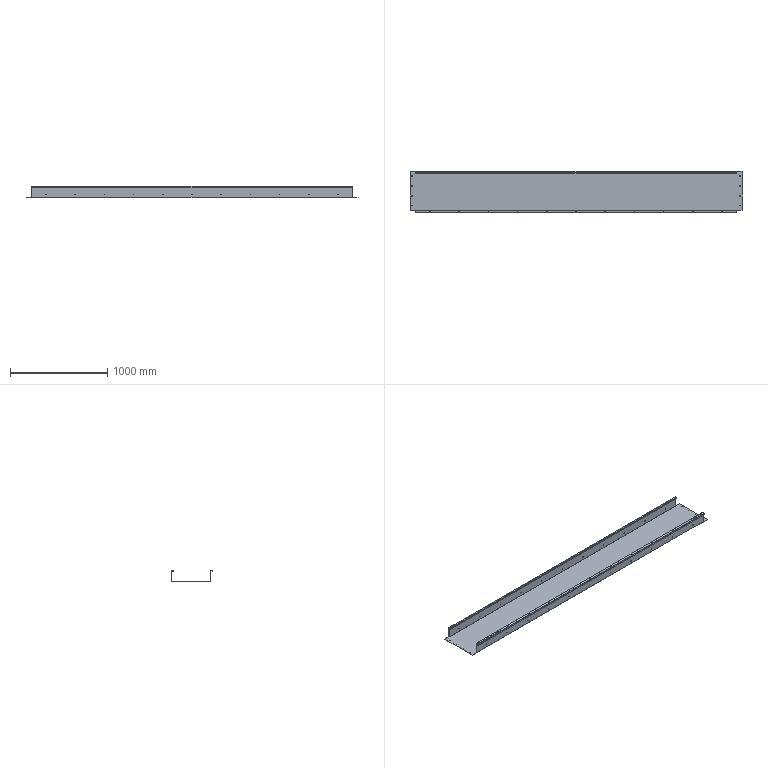Part | STEP file | TS-S94 | 1 solid | 196 faces | box 3411 x 423 x 122 mm | volume 4691933 mm3 | cylinder 116 | plane 80 | commonest cylinder face diameters 5.4 x66 8 x22 7 x16 0.4 x6 4.4 x6